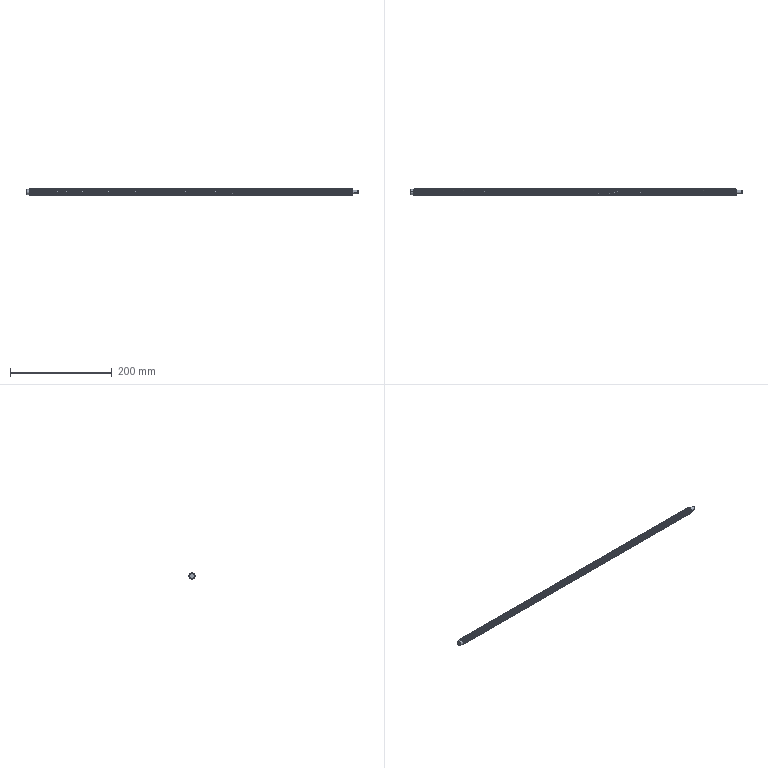Part | Creo | features CURVE 3, CUT 3, DATUM PLANE 3, CHAMFER 1, COORDINATE SYSTEM 1, PROTRUSION 1 | 1 solid | 489 faces | volume 61119 mm3 | cylinder 426 | spline 54 | cone 5 | plane 4 | commonest cylinder face diameters 12 x422 7 x2 10 x2